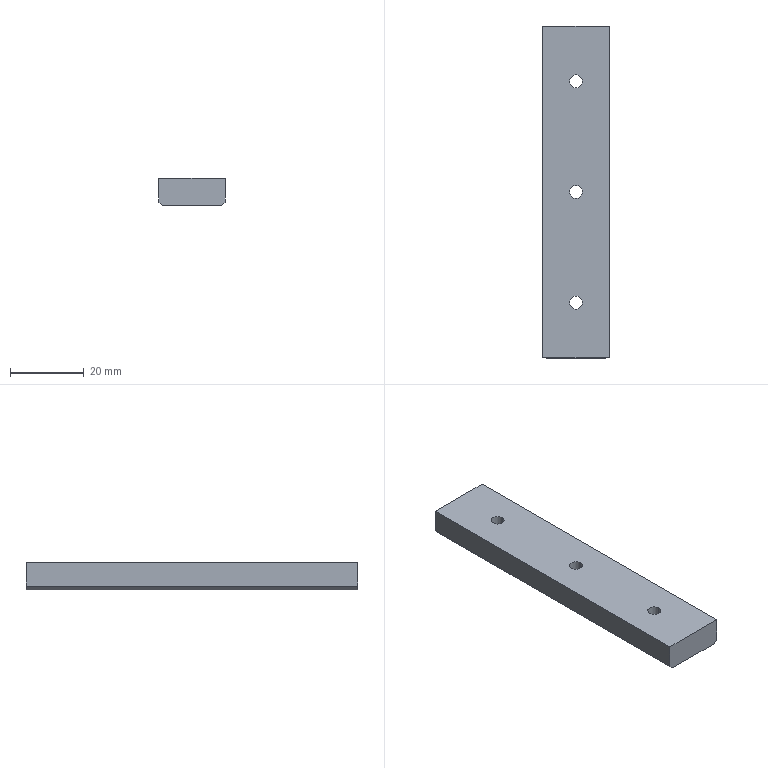Part | SolidWorks | features ICE 2, LPattern 2, Chamfer 1, Extrusion 1 | 1 solid | 23 faces | box 18 x 90 x 7.5 mm | volume 11592 mm3 | cylinder 12 | plane 11 | commonest cylinder face diameters 3.5 x6 6 x6
STEP:
#1=CARTESIAN_POINT('',(1.75,75.,3.75));
#2=VERTEX_POINT('',#1);
#3=CARTESIAN_POINT('',(-1.75,75.,3.75));
#4=VERTEX_POINT('',#3);
#5=CARTESIAN_POINT('',(0.,75.,3.75));
#6=DIRECTION('',(0.,0.,-1.));
#7=DIRECTION('',(-1.,0.,0.));
#8=AXIS2_PLACEMENT_3D('',#5,#6,#7);
#9=CIRCLE('',#8,1.75);
#10=EDGE_CURVE('',#2,#4,#9,.T.);
#11=ORIENTED_EDGE('',*,*,#10,.F.);
#12=CARTESIAN_POINT('',(1.75,75.,0.75));
#13=VERTEX_POINT('',#12);
#14=CARTESIAN_POINT('',(1.75,75.,3.75));
#15=DIRECTION('',(0.,0.,-1.));
#16=VECTOR('',#15,1000.);
#17=LINE('',#14,#16);
#18=EDGE_CURVE('',#2,#13,#17,.T.);
#19=ORIENTED_EDGE('',*,*,#18,.T.);
#20=CARTESIAN_POINT('',(-1.75,75.,0.75));
#21=VERTEX_POINT('',#20);
#22=CARTESIAN_POINT('',(0.,75.,0.75));
#23=DIRECTION('',(0.,0.,-1.));
#24=DIRECTION('',(-1.,0.,0.));
#25=AXIS2_PLACEMENT_3D('',#22,#23,#24);
#26=CIRCLE('',#25,1.75);
#27=EDGE_CURVE('',#13,#21,#26,.T.);
#28=ORIENTED_EDGE('',*,*,#27,.T.);
#29=CARTESIAN_POINT('',(-1.75,75.,3.75));
#30=DIRECTION('',(0.,0.,-1.));
#31=VECTOR('',#30,1000.);
#32=LINE('',#29,#31);
#33=EDGE_CURVE('',#4,#21,#32,.T.);
#34=ORIENTED_EDGE('',*,*,#33,.F.);
#35=EDGE_LOOP('',(#11,#19,#28,#34));
#36=FACE_OUTER_BOUND('',#35,.T.);
#37=CARTESIAN_POINT('',(0.,75.,3.75));
#38=DIRECTION('',(0.,0.,-1.));
#39=DIRECTION('',(-1.,0.,0.));
#40=AXIS2_PLACEMENT_3D('',#37,#38,#39);
#41=CYLINDRICAL_SURFACE('',#40,1.75);
#42=ADVANCED_FACE('',(#36),#41,.F.);
#43=CARTESIAN_POINT('',(1.75,45.,3.75));
#44=VERTEX_POINT('',#43);
#45=CARTESIAN_POINT('',(-1.75,45.,3.75));
#46=VERTEX_POINT('',#45);
#47=CARTESIAN_POINT('',(0.,45.,3.75));
#48=DIRECTION('',(0.,0.,-1.));
#49=DIRECTION('',(-1.,0.,0.));
#50=AXIS2_PLACEMENT_3D('',#47,#48,#49);
#51=CIRCLE('',#50,1.75);
#52=EDGE_CURVE('',#44,#46,#51,.T.);
#53=ORIENTED_EDGE('',*,*,#52,.F.);
#54=CARTESIAN_POINT('',(1.75,45.,0.75));
#55=VERTEX_POINT('',#54);
#56=CARTESIAN_POINT('',(1.75,45.,3.75));
#57=DIRECTION('',(0.,0.,-1.));
#58=VECTOR('',#57,1000.);
#59=LINE('',#56,#58);
#60=EDGE_CURVE('',#44,#55,#59,.T.);
#61=ORIENTED_EDGE('',*,*,#60,.T.);
#62=CARTESIAN_POINT('',(-1.75,45.,0.75));
#63=VERTEX_POINT('',#62);
#64=CARTESIAN_POINT('',(0.,45.,0.75));
#65=DIRECTION('',(0.,0.,-1.));
#66=DIRECTION('',(-1.,0.,0.));
#67=AXIS2_PLACEMENT_3D('',#64,#65,#66);
#68=CIRCLE('',#67,1.75);
#69=EDGE_CURVE('',#55,#63,#68,.T.);
#70=ORIENTED_EDGE('',*,*,#69,.T.);
#71=CARTESIAN_POINT('',(-1.75,45.,3.75));
#72=DIRECTION('',(0.,0.,-1.));
#73=VECTOR('',#72,1000.);
#74=LINE('',#71,#73);
#75=EDGE_CURVE('',#46,#63,#74,.T.);
#76=ORIENTED_EDGE('',*,*,#75,.F.);
#77=EDGE_LOOP('',(#53,#61,#70,#76));
#78=FACE_OUTER_BOUND('',#77,.T.);
#79=CARTESIAN_POINT('',(0.,45.,3.75));
#80=DIRECTION('',(0.,0.,-1.));
#81=DIRECTION('',(-1.,0.,0.));
#82=AXIS2_PLACEMENT_3D('',#79,#80,#81);
#83=CYLINDRICAL_SURFACE('',#82,1.75);
#84=ADVANCED_FACE('',(#78),#83,.F.);
#85=CARTESIAN_POINT('',(3.,75.,0.75));
#86=VERTEX_POINT('',#85);
#87=CARTESIAN_POINT('',(-3.,75.,0.75));
#88=VERTEX_POINT('',#87);
#89=CARTESIAN_POINT('',(0.,75.,0.75));
#90=DIRECTION('',(0.,0.,-1.));
#91=DIRECTION('',(-1.,0.,0.));
#92=AXIS2_PLACEMENT_3D('',#89,#90,#91);
#93=CIRCLE('',#92,3.);
#94=EDGE_CURVE('',#86,#88,#93,.T.);
#95=ORIENTED_EDGE('',*,*,#94,.F.);
#96=CARTESIAN_POINT('',(3.,75.,-3.75));
#97=VERTEX_POINT('',#96);
#98=CARTESIAN_POINT('',(3.,75.,0.75));
#99=DIRECTION('',(0.,0.,-1.));
#100=VECTOR('',#99,1000.);
#101=LINE('',#98,#100);
#102=EDGE_CURVE('',#86,#97,#101,.T.);
#103=ORIENTED_EDGE('',*,*,#102,.T.);
#104=CARTESIAN_POINT('',(-3.,75.,-3.75));
#105=VERTEX_POINT('',#104);
#106=CARTESIAN_POINT('',(0.,75.,-3.75));
#107=DIRECTION('',(0.,0.,-1.));
#108=DIRECTION('',(-1.,0.,0.));
#109=AXIS2_PLACEMENT_3D('',#106,#107,#108);
#110=CIRCLE('',#109,3.);
#111=EDGE_CURVE('',#97,#105,#110,.T.);
#112=ORIENTED_EDGE('',*,*,#111,.T.);
#113=CARTESIAN_POINT('',(-3.,75.,0.75));
#114=DIRECTION('',(0.,0.,-1.));
#115=VECTOR('',#114,1000.);
#116=LINE('',#113,#115);
#117=EDGE_CURVE('',#88,#105,#116,.T.);
#118=ORIENTED_EDGE('',*,*,#117,.F.);
#119=EDGE_LOOP('',(#95,#103,#112,#118));
#120=FACE_OUTER_BOUND('',#119,.T.);
#121=CARTESIAN_POINT('',(0.,75.,0.75));
#122=DIRECTION('',(0.,0.,-1.));
#123=DIRECTION('',(-1.,0.,0.));
#124=AXIS2_PLACEMENT_3D('',#121,#122,#123);
#125=CYLINDRICAL_SURFACE('',#124,3.);
#126=ADVANCED_FACE('',(#120),#125,.F.);
#127=CARTESIAN_POINT('',(3.,45.,0.75));
#128=VERTEX_POINT('',#127);
#129=CARTESIAN_POINT('',(-3.,45.,0.75));
#130=VERTEX_POINT('',#129);
#131=CARTESIAN_POINT('',(0.,45.,0.75));
#132=DIRECTION('',(0.,0.,-1.));
#133=DIRECTION('',(-1.,0.,0.));
#134=AXIS2_PLACEMENT_3D('',#131,#132,#133);
#135=CIRCLE('',#134,3.);
#136=EDGE_CURVE('',#128,#130,#135,.T.);
#137=ORIENTED_EDGE('',*,*,#136,.F.);
#138=CARTESIAN_POINT('',(3.,45.,-3.75));
#139=VERTEX_POINT('',#138);
#140=CARTESIAN_POINT('',(3.,45.,0.75));
#141=DIRECTION('',(0.,0.,-1.));
#142=VECTOR('',#141,1000.);
#143=LINE('',#140,#142);
#144=EDGE_CURVE('',#128,#139,#143,.T.);
#145=ORIENTED_EDGE('',*,*,#144,.T.);
#146=CARTESIAN_POINT('',(-3.,45.,-3.75));
#147=VERTEX_POINT('',#146);
#148=CARTESIAN_POINT('',(0.,45.,-3.75));
#149=DIRECTION('',(0.,0.,-1.));
#150=DIRECTION('',(-1.,0.,0.));
#151=AXIS2_PLACEMENT_3D('',#148,#149,#150);
#152=CIRCLE('',#151,3.);
#153=EDGE_CURVE('',#139,#147,#152,.T.);
#154=ORIENTED_EDGE('',*,*,#153,.T.);
#155=CARTESIAN_POINT('',(-3.,45.,0.75));
#156=DIRECTION('',(0.,0.,-1.));
#157=VECTOR('',#156,1000.);
#158=LINE('',#155,#157);
#159=EDGE_CURVE('',#130,#147,#158,.T.);
#160=ORIENTED_EDGE('',*,*,#159,.F.);
#161=EDGE_LOOP('',(#137,#145,#154,#160));
#162=FACE_OUTER_BOUND('',#161,.T.);
#163=CARTESIAN_POINT('',(0.,45.,0.75));
#164=DIRECTION('',(0.,0.,-1.));
#165=DIRECTION('',(-1.,0.,0.));
#166=AXIS2_PLACEMENT_3D('',#163,#164,#165);
#167=CYLINDRICAL_SURFACE('',#166,3.);
#168=ADVANCED_FACE('',(#162),#167,.F.);
#169=CARTESIAN_POINT('',(3.,15.,0.75));
#170=VERTEX_POINT('',#169);
#171=CARTESIAN_POINT('',(-3.,15.,0.75));
#172=VERTEX_POINT('',#171);
#173=CARTESIAN_POINT('',(0.,15.,0.75));
#174=DIRECTION('',(0.,0.,-1.));
#175=DIRECTION('',(-1.,0.,0.));
#176=AXIS2_PLACEMENT_3D('',#173,#174,#175);
#177=CIRCLE('',#176,3.);
#178=EDGE_CURVE('',#170,#172,#177,.T.);
#179=ORIENTED_EDGE('',*,*,#178,.F.);
#180=CARTESIAN_POINT('',(3.,15.,-3.75));
#181=VERTEX_POINT('',#180);
#182=CARTESIAN_POINT('',(3.,15.,0.75));
#183=DIRECTION('',(0.,0.,-1.));
#184=VECTOR('',#183,1000.);
#185=LINE('',#182,#184);
#186=EDGE_CURVE('',#170,#181,#185,.T.);
#187=ORIENTED_EDGE('',*,*,#186,.T.);
#188=CARTESIAN_POINT('',(-3.,15.,-3.75));
#189=VERTEX_POINT('',#188);
#190=CARTESIAN_POINT('',(0.,15.,-3.75));
#191=DIRECTION('',(0.,0.,-1.));
#192=DIRECTION('',(-1.,0.,0.));
#193=AXIS2_PLACEMENT_3D('',#190,#191,#192);
#194=CIRCLE('',#193,3.);
#195=EDGE_CURVE('',#181,#189,#194,.T.);
#196=ORIENTED_EDGE('',*,*,#195,.T.);
#197=CARTESIAN_POINT('',(-3.,15.,0.75));
#198=DIRECTION('',(0.,0.,-1.));
#199=VECTOR('',#198,1000.);
#200=LINE('',#197,#199);
#201=EDGE_CURVE('',#172,#189,#200,.T.);
#202=ORIENTED_EDGE('',*,*,#201,.F.);
#203=EDGE_LOOP('',(#179,#187,#196,#202));
#204=FACE_OUTER_BOUND('',#203,.T.);
#205=CARTESIAN_POINT('',(0.,15.,0.75));
#206=DIRECTION('',(0.,0.,-1.));
#207=DIRECTION('',(-1.,0.,0.));
#208=AXIS2_PLACEMENT_3D('',#205,#206,#207);
#209=CYLINDRICAL_SURFACE('',#208,3.);
#210=ADVANCED_FACE('',(#204),#209,.F.);
#211=CARTESIAN_POINT('',(1.75,15.,3.75));
#212=VERTEX_POINT('',#211);
#213=CARTESIAN_POINT('',(-1.75,15.,3.75));
#214=VERTEX_POINT('',#213);
#215=CARTESIAN_POINT('',(0.,15.,3.75));
#216=DIRECTION('',(0.,0.,-1.));
#217=DIRECTION('',(-1.,0.,0.));
#218=AXIS2_PLACEMENT_3D('',#215,#216,#217);
#219=CIRCLE('',#218,1.75);
#220=EDGE_CURVE('',#212,#214,#219,.T.);
#221=ORIENTED_EDGE('',*,*,#220,.F.);
#222=CARTESIAN_POINT('',(1.75,15.,0.75));
#223=VERTEX_POINT('',#222);
#224=CARTESIAN_POINT('',(1.75,15.,3.75));
#225=DIRECTION('',(0.,0.,-1.));
#226=VECTOR('',#225,1000.);
#227=LINE('',#224,#226);
#228=EDGE_CURVE('',#212,#223,#227,.T.);
#229=ORIENTED_EDGE('',*,*,#228,.T.);
#230=CARTESIAN_POINT('',(-1.75,15.,0.75));
#231=VERTEX_POINT('',#230);
#232=CARTESIAN_POINT('',(0.,15.,0.75));
#233=DIRECTION('',(0.,0.,1.));
#234=DIRECTION('',(-1.,0.,0.));
#235=AXIS2_PLACEMENT_3D('',#232,#233,#234);
#236=CIRCLE('',#235,1.75);
#237=EDGE_CURVE('',#231,#223,#236,.T.);
#238=ORIENTED_EDGE('',*,*,#237,.F.);
#239=CARTESIAN_POINT('',(-1.75,15.,3.75));
#240=DIRECTION('',(0.,0.,-1.));
#241=VECTOR('',#240,1000.);
#242=LINE('',#239,#241);
#243=EDGE_CURVE('',#214,#231,#242,.T.);
#244=ORIENTED_EDGE('',*,*,#243,.F.);
#245=EDGE_LOOP('',(#221,#229,#238,#244));
#246=FACE_OUTER_BOUND('',#245,.T.);
#247=CARTESIAN_POINT('',(0.,15.,3.75));
#248=DIRECTION('',(0.,0.,-1.));
#249=DIRECTION('',(-1.,0.,0.));
#250=AXIS2_PLACEMENT_3D('',#247,#248,#249);
#251=CYLINDRICAL_SURFACE('',#250,1.75);
#252=ADVANCED_FACE('',(#246),#251,.F.);
#253=ORIENTED_EDGE('',*,*,#228,.F.);
#254=CARTESIAN_POINT('',(0.,15.,3.75));
#255=DIRECTION('',(0.,0.,-1.));
#256=DIRECTION('',(-1.,0.,0.));
#257=AXIS2_PLACEMENT_3D('',#254,#255,#256);
#258=CIRCLE('',#257,1.75);
#259=EDGE_CURVE('',#214,#212,#258,.T.);
#260=ORIENTED_EDGE('',*,*,#259,.F.);
#261=ORIENTED_EDGE('',*,*,#243,.T.);
#262=CARTESIAN_POINT('',(0.,15.,0.75));
#263=DIRECTION('',(0.,0.,1.));
#264=DIRECTION('',(-1.,0.,0.));
#265=AXIS2_PLACEMENT_3D('',#262,#263,#264);
#266=CIRCLE('',#265,1.75);
#267=EDGE_CURVE('',#223,#231,#266,.T.);
#268=ORIENTED_EDGE('',*,*,#267,.F.);
#269=EDGE_LOOP('',(#253,#260,#261,#268));
#270=FACE_OUTER_BOUND('',#269,.T.);
#271=CARTESIAN_POINT('',(0.,15.,3.75));
#272=DIRECTION('',(0.,0.,-1.));
#273=DIRECTION('',(-1.,0.,0.));
#274=AXIS2_PLACEMENT_3D('',#271,#272,#273);
#275=CYLINDRICAL_SURFACE('',#274,1.75);
#276=ADVANCED_FACE('',(#270),#275,.F.);
#277=CARTESIAN_POINT('',(9.,0.,3.75));
#278=VERTEX_POINT('',#277);
#279=CARTESIAN_POINT('',(9.,0.,-2.75));
#280=VERTEX_POINT('',#279);
#281=CARTESIAN_POINT('',(9.,0.,-3.75));
#282=DIRECTION('',(0.,0.,-1.));
#283=VECTOR('',#282,1000.);
#284=LINE('',#281,#283);
#285=EDGE_CURVE('',#278,#280,#284,.T.);
#286=ORIENTED_EDGE('',*,*,#285,.T.);
#287=CARTESIAN_POINT('',(9.,90.,-2.75));
#288=VERTEX_POINT('',#287);
#289=CARTESIAN_POINT('',(9.,90.,-2.75));
#290=DIRECTION('',(0.,1.,0.));
#291=VECTOR('',#290,1000.);
#292=LINE('',#289,#291);
#293=EDGE_CURVE('',#280,#288,#292,.T.);
#294=ORIENTED_EDGE('',*,*,#293,.T.);
#295=CARTESIAN_POINT('',(9.,90.,3.75));
#296=VERTEX_POINT('',#295);
#297=CARTESIAN_POINT('',(9.,90.,-3.75));
#298=DIRECTION('',(0.,0.,-1.));
#299=VECTOR('',#298,1000.);
#300=LINE('',#297,#299);
#301=EDGE_CURVE('',#296,#288,#300,.T.);
#302=ORIENTED_EDGE('',*,*,#301,.F.);
#303=CARTESIAN_POINT('',(9.,90.,3.75));
#304=DIRECTION('',(0.,-1.,0.));
#305=VECTOR('',#304,1000.);
#306=LINE('',#303,#305);
#307=EDGE_CURVE('',#296,#278,#306,.T.);
#308=ORIENTED_EDGE('',*,*,#307,.T.);
#309=EDGE_LOOP('',(#286,#294,#302,#308));
#310=FACE_OUTER_BOUND('',#309,.T.);
#311=CARTESIAN_POINT('',(9.,90.,-3.75));
#312=DIRECTION('',(-1.,0.,0.));
#313=DIRECTION('',(0.,0.,1.));
#314=AXIS2_PLACEMENT_3D('',#311,#312,#313);
#315=PLANE('',#314);
#316=ADVANCED_FACE('',(#310),#315,.F.);
#317=CARTESIAN_POINT('',(0.,75.,-3.75));
#318=DIRECTION('',(0.,0.,-1.));
#319=DIRECTION('',(-1.,0.,0.));
#320=AXIS2_PLACEMENT_3D('',#317,#318,#319);
#321=CIRCLE('',#320,3.);
#322=EDGE_CURVE('',#105,#97,#321,.T.);
#323=ORIENTED_EDGE('',*,*,#322,.F.);
#324=ORIENTED_EDGE('',*,*,#111,.F.);
#325=EDGE_LOOP('',(#323,#324));
#326=FACE_BOUND('',#325,.T.);
#327=CARTESIAN_POINT('',(0.,45.,-3.75));
#328=DIRECTION('',(0.,0.,-1.));
#329=DIRECTION('',(-1.,0.,0.));
#330=AXIS2_PLACEMENT_3D('',#327,#328,#329);
#331=CIRCLE('',#330,3.);
#332=EDGE_CURVE('',#147,#139,#331,.T.);
#333=ORIENTED_EDGE('',*,*,#332,.F.);
#334=ORIENTED_EDGE('',*,*,#153,.F.);
#335=EDGE_LOOP('',(#333,#334));
#336=FACE_BOUND('',#335,.T.);
#337=CARTESIAN_POINT('',(0.,15.,-3.75));
#338=DIRECTION('',(0.,0.,-1.));
#339=DIRECTION('',(-1.,0.,0.));
#340=AXIS2_PLACEMENT_3D('',#337,#338,#339);
#341=CIRCLE('',#340,3.);
#342=EDGE_CURVE('',#189,#181,#341,.T.);
#343=ORIENTED_EDGE('',*,*,#342,.F.);
#344=ORIENTED_EDGE('',*,*,#195,.F.);
#345=EDGE_LOOP('',(#343,#344));
#346=FACE_BOUND('',#345,.T.);
#347=CARTESIAN_POINT('',(8.,0.,-3.75));
#348=VERTEX_POINT('',#347);
#349=CARTESIAN_POINT('',(-8.,0.,-3.75));
#350=VERTEX_POINT('',#349);
#351=CARTESIAN_POINT('',(-9.,0.,-3.75));
#352=DIRECTION('',(-1.,0.,0.));
#353=VECTOR('',#352,1000.);
#354=LINE('',#351,#353);
#355=EDGE_CURVE('',#348,#350,#354,.T.);
#356=ORIENTED_EDGE('',*,*,#355,.T.);
#357=CARTESIAN_POINT('',(-8.,90.,-3.75));
#358=VERTEX_POINT('',#357);
#359=CARTESIAN_POINT('',(-8.,90.,-3.75));
#360=DIRECTION('',(0.,1.,0.));
#361=VECTOR('',#360,1000.);
#362=LINE('',#359,#361);
#363=EDGE_CURVE('',#350,#358,#362,.T.);
#364=ORIENTED_EDGE('',*,*,#363,.T.);
#365=CARTESIAN_POINT('',(8.,90.,-3.75));
#366=VERTEX_POINT('',#365);
#367=CARTESIAN_POINT('',(-9.,90.,-3.75));
#368=DIRECTION('',(-1.,0.,0.));
#369=VECTOR('',#368,1000.);
#370=LINE('',#367,#369);
#371=EDGE_CURVE('',#366,#358,#370,.T.);
#372=ORIENTED_EDGE('',*,*,#371,.F.);
#373=CARTESIAN_POINT('',(8.,90.,-3.75));
#374=DIRECTION('',(0.,-1.,0.));
#375=VECTOR('',#374,1000.);
#376=LINE('',#373,#375);
#377=EDGE_CURVE('',#366,#348,#376,.T.);
#378=ORIENTED_EDGE('',*,*,#377,.T.);
#379=EDGE_LOOP('',(#356,#364,#372,#378));
#380=FACE_OUTER_BOUND('',#379,.T.);
#381=CARTESIAN_POINT('',(-9.,90.,-3.75));
#382=DIRECTION('',(0.,0.,1.));
#383=DIRECTION('',(1.,0.,0.));
#384=AXIS2_PLACEMENT_3D('',#381,#382,#383);
#385=PLANE('',#384);
#386=ADVANCED_FACE('',(#326,#336,#346,#380),#385,.F.);
#387=CARTESIAN_POINT('',(-9.,90.,-2.75));
#388=VERTEX_POINT('',#387);
#389=CARTESIAN_POINT('',(-9.,90.,3.75));
#390=VERTEX_POINT('',#389);
#391=CARTESIAN_POINT('',(-9.,90.,-3.75));
#392=DIRECTION('',(0.,0.,1.));
#393=VECTOR('',#392,1000.);
#394=LINE('',#391,#393);
#395=EDGE_CURVE('',#388,#390,#394,.T.);
#396=ORIENTED_EDGE('',*,*,#395,.F.);
#397=CARTESIAN_POINT('',(-9.,0.,-2.75));
#398=VERTEX_POINT('',#397);
#399=CARTESIAN_POINT('',(-9.,90.,-2.75));
#400=DIRECTION('',(0.,-1.,0.));
#401=VECTOR('',#400,1000.);
#402=LINE('',#399,#401);
#403=EDGE_CURVE('',#388,#398,#402,.T.);
#404=ORIENTED_EDGE('',*,*,#403,.T.);
#405=CARTESIAN_POINT('',(-9.,0.,3.75));
#406=VERTEX_POINT('',#405);
#407=CARTESIAN_POINT('',(-9.,0.,-3.75));
#408=DIRECTION('',(0.,0.,1.));
#409=VECTOR('',#408,1000.);
#410=LINE('',#407,#409);
#411=EDGE_CURVE('',#398,#406,#410,.T.);
#412=ORIENTED_EDGE('',*,*,#411,.T.);
#413=CARTESIAN_POINT('',(-9.,90.,3.75));
#414=DIRECTION('',(0.,-1.,0.));
#415=VECTOR('',#414,1000.);
#416=LINE('',#413,#415);
#417=EDGE_CURVE('',#390,#406,#416,.T.);
#418=ORIENTED_EDGE('',*,*,#417,.F.);
#419=EDGE_LOOP('',(#396,#404,#412,#418));
#420=FACE_OUTER_BOUND('',#419,.T.);
#421=CARTESIAN_POINT('',(-9.,90.,-3.75));
#422=DIRECTION('',(1.,0.,0.));
#423=DIRECTION('',(0.,0.,-1.));
#424=AXIS2_PLACEMENT_3D('',#421,#422,#423);
#425=PLANE('',#424);
#426=ADVANCED_FACE('',(#420),#425,.F.);
#427=CARTESIAN_POINT('',(0.,75.,3.75));
#428=DIRECTION('',(0.,0.,-1.));
#429=DIRECTION('',(-1.,0.,0.));
#430=AXIS2_PLACEMENT_3D('',#427,#428,#429);
#431=CIRCLE('',#430,1.75);
#432=EDGE_CURVE('',#4,#2,#431,.T.);
#433=ORIENTED_EDGE('',*,*,#432,.T.);
#434=ORIENTED_EDGE('',*,*,#10,.T.);
#435=EDGE_LOOP('',(#433,#434));
#436=FACE_BOUND('',#435,.T.);
#437=CARTESIAN_POINT('',(0.,45.,3.75));
#438=DIRECTION('',(0.,0.,-1.));
#439=DIRECTION('',(-1.,0.,0.));
#440=AXIS2_PLACEMENT_3D('',#437,#438,#439);
#441=CIRCLE('',#440,1.75);
#442=EDGE_CURVE('',#46,#44,#441,.T.);
#443=ORIENTED_EDGE('',*,*,#442,.T.);
#444=ORIENTED_EDGE('',*,*,#52,.T.);
#445=EDGE_LOOP('',(#443,#444));
#446=FACE_BOUND('',#445,.T.);
#447=ORIENTED_EDGE('',*,*,#259,.T.);
#448=ORIENTED_EDGE('',*,*,#220,.T.);
#449=EDGE_LOOP('',(#447,#448));
#450=FACE_BOUND('',#449,.T.);
#451=CARTESIAN_POINT('',(-9.,0.,3.75));
#452=DIRECTION('',(1.,0.,0.));
#453=VECTOR('',#452,1000.);
#454=LINE('',#451,#453);
#455=EDGE_CURVE('',#406,#278,#454,.T.);
#456=ORIENTED_EDGE('',*,*,#455,.T.);
#457=ORIENTED_EDGE('',*,*,#307,.F.);
#458=CARTESIAN_POINT('',(-9.,90.,3.75));
#459=DIRECTION('',(1.,0.,0.));
#460=VECTOR('',#459,1000.);
#461=LINE('',#458,#460);
#462=EDGE_CURVE('',#390,#296,#461,.T.);
#463=ORIENTED_EDGE('',*,*,#462,.F.);
#464=ORIENTED_EDGE('',*,*,#417,.T.);
#465=EDGE_LOOP('',(#456,#457,#463,#464));
#466=FACE_OUTER_BOUND('',#465,.T.);
#467=CARTESIAN_POINT('',(-9.,90.,3.75));
#468=DIRECTION('',(0.,0.,-1.));
#469=DIRECTION('',(-1.,0.,0.));
#470=AXIS2_PLACEMENT_3D('',#467,#468,#469);
#471=PLANE('',#470);
#472=ADVANCED_FACE('',(#436,#446,#450,#466),#471,.F.);
#473=ORIENTED_EDGE('',*,*,#371,.T.);
#474=CARTESIAN_POINT('',(-5.875,90.,-5.875));
#475=DIRECTION('',(-0.7071,0.,0.7071));
#476=VECTOR('',#475,1000.);
#477=LINE('',#474,#476);
#478=EDGE_CURVE('',#358,#388,#477,.T.);
#479=ORIENTED_EDGE('',*,*,#478,.T.);
#480=ORIENTED_EDGE('',*,*,#395,.T.);
#481=ORIENTED_EDGE('',*,*,#462,.T.);
#482=ORIENTED_EDGE('',*,*,#301,.T.);
#483=CARTESIAN_POINT('',(5.875,90.,-5.875));
#484=DIRECTION('',(-0.7071,0.,-0.7071));
#485=VECTOR('',#484,1000.);
#486=LINE('',#483,#485);
#487=EDGE_CURVE('',#288,#366,#486,.T.);
#488=ORIENTED_EDGE('',*,*,#487,.T.);
#489=EDGE_LOOP('',(#473,#479,#480,#481,#482,#488));
#490=FACE_OUTER_BOUND('',#489,.T.);
#491=CARTESIAN_POINT('',(0.,90.,0.));
#492=DIRECTION('',(0.,1.,0.));
#493=DIRECTION('',(0.,0.,1.));
#494=AXIS2_PLACEMENT_3D('',#491,#492,#493);
#495=PLANE('',#494);
#496=ADVANCED_FACE('',(#490),#495,.T.);
#497=ORIENTED_EDGE('',*,*,#411,.F.);
#498=CARTESIAN_POINT('',(-9.,0.,-2.75));
#499=DIRECTION('',(0.7071,0.,-0.7071));
#500=VECTOR('',#499,1000.);
#501=LINE('',#498,#500);
#502=EDGE_CURVE('',#398,#350,#501,.T.);
#503=ORIENTED_EDGE('',*,*,#502,.T.);
#504=ORIENTED_EDGE('',*,*,#355,.F.);
#505=CARTESIAN_POINT('',(8.,0.,-3.75));
#506=DIRECTION('',(0.7071,0.,0.7071));
#507=VECTOR('',#506,1000.);
#508=LINE('',#505,#507);
#509=EDGE_CURVE('',#348,#280,#508,.T.);
#510=ORIENTED_EDGE('',*,*,#509,.T.);
#511=ORIENTED_EDGE('',*,*,#285,.F.);
#512=ORIENTED_EDGE('',*,*,#455,.F.);
#513=EDGE_LOOP('',(#497,#503,#504,#510,#511,#512));
#514=FACE_OUTER_BOUND('',#513,.T.);
#515=CARTESIAN_POINT('',(0.,0.,0.));
#516=DIRECTION('',(0.,1.,0.));
#517=DIRECTION('',(0.,0.,1.));
#518=AXIS2_PLACEMENT_3D('',#515,#516,#517);
#519=PLANE('',#518);
#520=ADVANCED_FACE('',(#514),#519,.F.);
#521=ORIENTED_EDGE('',*,*,#478,.F.);
#522=ORIENTED_EDGE('',*,*,#363,.F.);
#523=ORIENTED_EDGE('',*,*,#502,.F.);
#524=ORIENTED_EDGE('',*,*,#403,.F.);
#525=EDGE_LOOP('',(#521,#522,#523,#524));
#526=FACE_OUTER_BOUND('',#525,.T.);
#527=CARTESIAN_POINT('',(-9.,90.,-2.75));
#528=DIRECTION('',(0.7071,0.,0.7071));
#529=DIRECTION('',(0.,-1.,0.));
#530=AXIS2_PLACEMENT_3D('',#527,#528,#529);
#531=PLANE('',#530);
#532=ADVANCED_FACE('',(#526),#531,.F.);
#533=ORIENTED_EDGE('',*,*,#487,.F.);
#534=ORIENTED_EDGE('',*,*,#293,.F.);
#535=ORIENTED_EDGE('',*,*,#509,.F.);
#536=ORIENTED_EDGE('',*,*,#377,.F.);
#537=EDGE_LOOP('',(#533,#534,#535,#536));
#538=FACE_OUTER_BOUND('',#537,.T.);
#539=CARTESIAN_POINT('',(8.,90.,-3.75));
#540=DIRECTION('',(-0.7071,0.,0.7071));
#541=DIRECTION('',(0.,-1.,0.));
#542=AXIS2_PLACEMENT_3D('',#539,#540,#541);
#543=PLANE('',#542);
#544=ADVANCED_FACE('',(#538),#543,.F.);
#545=CARTESIAN_POINT('',(0.,15.,0.75));
#546=DIRECTION('',(0.,0.,-1.));
#547=DIRECTION('',(-1.,0.,0.));
#548=AXIS2_PLACEMENT_3D('',#545,#546,#547);
#549=CIRCLE('',#548,3.);
#550=EDGE_CURVE('',#172,#170,#549,.T.);
#551=ORIENTED_EDGE('',*,*,#550,.T.);
#552=ORIENTED_EDGE('',*,*,#178,.T.);
#553=EDGE_LOOP('',(#551,#552));
#554=FACE_OUTER_BOUND('',#553,.T.);
#555=ORIENTED_EDGE('',*,*,#237,.T.);
#556=ORIENTED_EDGE('',*,*,#267,.T.);
#557=EDGE_LOOP('',(#555,#556));
#558=FACE_BOUND('',#557,.T.);
#559=CARTESIAN_POINT('',(0.,15.,0.75));
#560=DIRECTION('',(0.,0.,-1.));
#561=DIRECTION('',(-1.,0.,0.));
#562=AXIS2_PLACEMENT_3D('',#559,#560,#561);
#563=PLANE('',#562);
#564=ADVANCED_FACE('',(#554,#558),#563,.T.);
#565=ORIENTED_EDGE('',*,*,#186,.F.);
#566=ORIENTED_EDGE('',*,*,#550,.F.);
#567=ORIENTED_EDGE('',*,*,#201,.T.);
#568=ORIENTED_EDGE('',*,*,#342,.T.);
#569=EDGE_LOOP('',(#565,#566,#567,#568));
#570=FACE_OUTER_BOUND('',#569,.T.);
#571=CARTESIAN_POINT('',(0.,15.,0.75));
#572=DIRECTION('',(0.,0.,-1.));
#573=DIRECTION('',(-1.,0.,0.));
#574=AXIS2_PLACEMENT_3D('',#571,#572,#573);
#575=CYLINDRICAL_SURFACE('',#574,3.);
#576=ADVANCED_FACE('',(#570),#575,.F.);
#577=ORIENTED_EDGE('',*,*,#144,.F.);
#578=CARTESIAN_POINT('',(0.,45.,0.75));
#579=DIRECTION('',(0.,0.,-1.));
#580=DIRECTION('',(-1.,0.,0.));
#581=AXIS2_PLACEMENT_3D('',#578,#579,#580);
#582=CIRCLE('',#581,3.);
#583=EDGE_CURVE('',#130,#128,#582,.T.);
#584=ORIENTED_EDGE('',*,*,#583,.F.);
#585=ORIENTED_EDGE('',*,*,#159,.T.);
#586=ORIENTED_EDGE('',*,*,#332,.T.);
#587=EDGE_LOOP('',(#577,#584,#585,#586));
#588=FACE_OUTER_BOUND('',#587,.T.);
#589=CARTESIAN_POINT('',(0.,45.,0.75));
#590=DIRECTION('',(0.,0.,-1.));
#591=DIRECTION('',(-1.,0.,0.));
#592=AXIS2_PLACEMENT_3D('',#589,#590,#591);
#593=CYLINDRICAL_SURFACE('',#592,3.);
#594=ADVANCED_FACE('',(#588),#593,.F.);
#595=CARTESIAN_POINT('',(0.,45.,0.75));
#596=DIRECTION('',(0.,0.,-1.));
#597=DIRECTION('',(-1.,0.,0.));
#598=AXIS2_PLACEMENT_3D('',#595,#596,#597);
#599=CIRCLE('',#598,1.75);
#600=EDGE_CURVE('',#63,#55,#599,.T.);
#601=ORIENTED_EDGE('',*,*,#600,.F.);
#602=ORIENTED_EDGE('',*,*,#69,.F.);
#603=EDGE_LOOP('',(#601,#602));
#604=FACE_BOUND('',#603,.T.);
#605=ORIENTED_EDGE('',*,*,#583,.T.);
#606=ORIENTED_EDGE('',*,*,#136,.T.);
#607=EDGE_LOOP('',(#605,#606));
#608=FACE_OUTER_BOUND('',#607,.T.);
#609=CARTESIAN_POINT('',(0.,45.,0.75));
#610=DIRECTION('',(0.,0.,-1.));
#611=DIRECTION('',(-1.,0.,0.));
#612=AXIS2_PLACEMENT_3D('',#609,#610,#611);
#613=PLANE('',#612);
#614=ADVANCED_FACE('',(#604,#608),#613,.T.);
#615=ORIENTED_EDGE('',*,*,#102,.F.);
#616=CARTESIAN_POINT('',(0.,75.,0.75));
#617=DIRECTION('',(0.,0.,-1.));
#618=DIRECTION('',(-1.,0.,0.));
#619=AXIS2_PLACEMENT_3D('',#616,#617,#618);
#620=CIRCLE('',#619,3.);
#621=EDGE_CURVE('',#88,#86,#620,.T.);
#622=ORIENTED_EDGE('',*,*,#621,.F.);
#623=ORIENTED_EDGE('',*,*,#117,.T.);
#624=ORIENTED_EDGE('',*,*,#322,.T.);
#625=EDGE_LOOP('',(#615,#622,#623,#624));
#626=FACE_OUTER_BOUND('',#625,.T.);
#627=CARTESIAN_POINT('',(0.,75.,0.75));
#628=DIRECTION('',(0.,0.,-1.));
#629=DIRECTION('',(-1.,0.,0.));
#630=AXIS2_PLACEMENT_3D('',#627,#628,#629);
#631=CYLINDRICAL_SURFACE('',#630,3.);
#632=ADVANCED_FACE('',(#626),#631,.F.);
#633=CARTESIAN_POINT('',(0.,75.,0.75));
#634=DIRECTION('',(0.,0.,-1.));
#635=DIRECTION('',(-1.,0.,0.));
#636=AXIS2_PLACEMENT_3D('',#633,#634,#635);
#637=CIRCLE('',#636,1.75);
#638=EDGE_CURVE('',#21,#13,#637,.T.);
#639=ORIENTED_EDGE('',*,*,#638,.F.);
#640=ORIENTED_EDGE('',*,*,#27,.F.);
#641=EDGE_LOOP('',(#639,#640));
#642=FACE_BOUND('',#641,.T.);
#643=ORIENTED_EDGE('',*,*,#621,.T.);
#644=ORIENTED_EDGE('',*,*,#94,.T.);
#645=EDGE_LOOP('',(#643,#644));
#646=FACE_OUTER_BOUND('',#645,.T.);
#647=CARTESIAN_POINT('',(0.,75.,0.75));
#648=DIRECTION('',(0.,0.,-1.));
#649=DIRECTION('',(-1.,0.,0.));
#650=AXIS2_PLACEMENT_3D('',#647,#648,#649);
#651=PLANE('',#650);
#652=ADVANCED_FACE('',(#642,#646),#651,.T.);
#653=ORIENTED_EDGE('',*,*,#60,.F.);
#654=ORIENTED_EDGE('',*,*,#442,.F.);
#655=ORIENTED_EDGE('',*,*,#75,.T.);
#656=ORIENTED_EDGE('',*,*,#600,.T.);
#657=EDGE_LOOP('',(#653,#654,#655,#656));
#658=FACE_OUTER_BOUND('',#657,.T.);
#659=CARTESIAN_POINT('',(0.,45.,3.75));
#660=DIRECTION('',(0.,0.,-1.));
#661=DIRECTION('',(-1.,0.,0.));
#662=AXIS2_PLACEMENT_3D('',#659,#660,#661);
#663=CYLINDRICAL_SURFACE('',#662,1.75);
#664=ADVANCED_FACE('',(#658),#663,.F.);
#665=ORIENTED_EDGE('',*,*,#18,.F.);
#666=ORIENTED_EDGE('',*,*,#432,.F.);
#667=ORIENTED_EDGE('',*,*,#33,.T.);
#668=ORIENTED_EDGE('',*,*,#638,.T.);
#669=EDGE_LOOP('',(#665,#666,#667,#668));
#670=FACE_OUTER_BOUND('',#669,.T.);
#671=CARTESIAN_POINT('',(0.,75.,3.75));
#672=DIRECTION('',(0.,0.,-1.));
#673=DIRECTION('',(-1.,0.,0.));
#674=AXIS2_PLACEMENT_3D('',#671,#672,#673);
#675=CYLINDRICAL_SURFACE('',#674,1.75);
#676=ADVANCED_FACE('',(#670),#675,.F.);
#677=CLOSED_SHELL('',(#42,#84,#126,#168,#210,#252,#276,#316,#386,#426,#472,#496,#520,#532,#544,#564,#576,#594,#614,#632,#652,#664,#676));
#678=MANIFOLD_SOLID_BREP('',#677);
#679=CARTESIAN_POINT('',(0.,0.,0.));
#680=DIRECTION('',(0.,0.,1.));
#681=DIRECTION('',(1.,0.,0.));
#682=AXIS2_PLACEMENT_3D('',#679,#680,#681);
#683=(LENGTH_UNIT()NAMED_UNIT(*)SI_UNIT(.MILLI.,.METRE.));
#684=UNCERTAINTY_MEASURE_WITH_UNIT(LENGTH_MEASURE(0.00001),#683,'','');
#685=(NAMED_UNIT(*)PLANE_ANGLE_UNIT()SI_UNIT($,.RADIAN.));
#686=(NAMED_UNIT(*)SI_UNIT($,.STERADIAN.)SOLID_ANGLE_UNIT());
#687=(GEOMETRIC_REPRESENTATION_CONTEXT(3)GLOBAL_UNCERTAINTY_ASSIGNED_CONTEXT((#684))GLOBAL_UNIT_ASSIGNED_CONTEXT((#683,#685,#686))REPRESENTATION_CONTEXT('',''));
#688=ADVANCED_BREP_SHAPE_REPRESENTATION('',(#678,#682),#687);